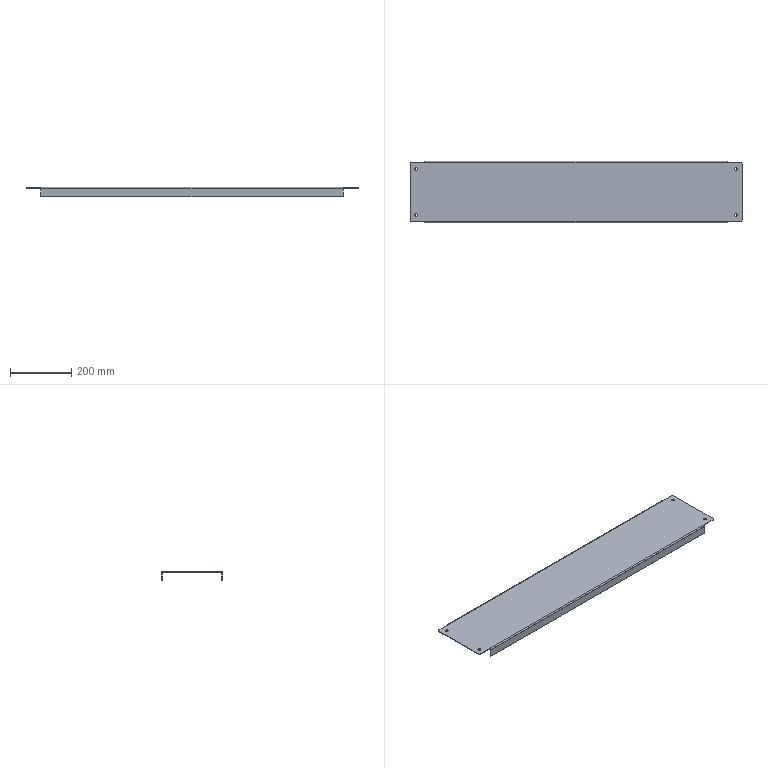Part | STEP file | 750038142 | 1 solid | 34 faces | box 1086 x 200 x 30 mm | volume 538093 mm3 | plane 18 | cylinder 16 | commonest cylinder face diameters 9 x8 10 x4 4 x2 8 x2
STEP:
#1=CARTESIAN_POINT('',(-527.5,-75.,0.));
#2=VERTEX_POINT('',#1);
#3=CARTESIAN_POINT('',(-518.5,-75.,0.));
#4=VERTEX_POINT('',#3);
#5=CARTESIAN_POINT('',(-523.,-75.,0.));
#6=DIRECTION('',(0.,0.,1.));
#7=DIRECTION('',(1.,0.,0.));
#8=AXIS2_PLACEMENT_3D('',#5,#6,#7);
#9=CIRCLE('',#8,4.5);
#10=EDGE_CURVE('',#2,#4,#9,.T.);
#11=ORIENTED_EDGE('',*,*,#10,.F.);
#12=CARTESIAN_POINT('',(-527.5,-75.,2.));
#13=VERTEX_POINT('',#12);
#14=CARTESIAN_POINT('',(-527.5,-75.,-1102.67));
#15=DIRECTION('',(0.,0.,1.));
#16=VECTOR('',#15,1000.);
#17=LINE('',#14,#16);
#18=EDGE_CURVE('',#2,#13,#17,.T.);
#19=ORIENTED_EDGE('',*,*,#18,.T.);
#20=CARTESIAN_POINT('',(-518.5,-75.,2.));
#21=VERTEX_POINT('',#20);
#22=CARTESIAN_POINT('',(-523.,-75.,2.));
#23=DIRECTION('',(0.,0.,-1.));
#24=DIRECTION('',(1.,0.,0.));
#25=AXIS2_PLACEMENT_3D('',#22,#23,#24);
#26=CIRCLE('',#25,4.5);
#27=EDGE_CURVE('',#21,#13,#26,.T.);
#28=ORIENTED_EDGE('',*,*,#27,.F.);
#29=CARTESIAN_POINT('',(-518.5,-75.,-1102.67));
#30=DIRECTION('',(0.,0.,1.));
#31=VECTOR('',#30,1000.);
#32=LINE('',#29,#31);
#33=EDGE_CURVE('',#4,#21,#32,.T.);
#34=ORIENTED_EDGE('',*,*,#33,.F.);
#35=EDGE_LOOP('',(#11,#19,#28,#34));
#36=FACE_OUTER_BOUND('',#35,.T.);
#37=CARTESIAN_POINT('',(-523.,-75.,-1102.67));
#38=DIRECTION('',(0.,0.,1.));
#39=DIRECTION('',(1.,0.,0.));
#40=AXIS2_PLACEMENT_3D('',#37,#38,#39);
#41=CYLINDRICAL_SURFACE('',#40,4.5);
#42=ADVANCED_FACE('',(#36),#41,.F.);
#43=CARTESIAN_POINT('',(-527.5,75.,0.));
#44=VERTEX_POINT('',#43);
#45=CARTESIAN_POINT('',(-518.5,75.,0.));
#46=VERTEX_POINT('',#45);
#47=CARTESIAN_POINT('',(-523.,75.,0.));
#48=DIRECTION('',(0.,0.,1.));
#49=DIRECTION('',(1.,0.,0.));
#50=AXIS2_PLACEMENT_3D('',#47,#48,#49);
#51=CIRCLE('',#50,4.5);
#52=EDGE_CURVE('',#44,#46,#51,.T.);
#53=ORIENTED_EDGE('',*,*,#52,.F.);
#54=CARTESIAN_POINT('',(-527.5,75.,2.));
#55=VERTEX_POINT('',#54);
#56=CARTESIAN_POINT('',(-527.5,75.,-1102.67));
#57=DIRECTION('',(0.,0.,1.));
#58=VECTOR('',#57,1000.);
#59=LINE('',#56,#58);
#60=EDGE_CURVE('',#44,#55,#59,.T.);
#61=ORIENTED_EDGE('',*,*,#60,.T.);
#62=CARTESIAN_POINT('',(-518.5,75.,2.));
#63=VERTEX_POINT('',#62);
#64=CARTESIAN_POINT('',(-523.,75.,2.));
#65=DIRECTION('',(0.,0.,-1.));
#66=DIRECTION('',(1.,0.,0.));
#67=AXIS2_PLACEMENT_3D('',#64,#65,#66);
#68=CIRCLE('',#67,4.5);
#69=EDGE_CURVE('',#63,#55,#68,.T.);
#70=ORIENTED_EDGE('',*,*,#69,.F.);
#71=CARTESIAN_POINT('',(-518.5,75.,-1102.67));
#72=DIRECTION('',(0.,0.,1.));
#73=VECTOR('',#72,1000.);
#74=LINE('',#71,#73);
#75=EDGE_CURVE('',#46,#63,#74,.T.);
#76=ORIENTED_EDGE('',*,*,#75,.F.);
#77=EDGE_LOOP('',(#53,#61,#70,#76));
#78=FACE_OUTER_BOUND('',#77,.T.);
#79=CARTESIAN_POINT('',(-523.,75.,-1102.67));
#80=DIRECTION('',(0.,0.,1.));
#81=DIRECTION('',(1.,0.,0.));
#82=AXIS2_PLACEMENT_3D('',#79,#80,#81);
#83=CYLINDRICAL_SURFACE('',#82,4.5);
#84=ADVANCED_FACE('',(#78),#83,.F.);
#85=CARTESIAN_POINT('',(518.5,-75.,0.));
#86=VERTEX_POINT('',#85);
#87=CARTESIAN_POINT('',(527.5,-75.,0.));
#88=VERTEX_POINT('',#87);
#89=CARTESIAN_POINT('',(523.,-75.,0.));
#90=DIRECTION('',(0.,0.,1.));
#91=DIRECTION('',(1.,0.,0.));
#92=AXIS2_PLACEMENT_3D('',#89,#90,#91);
#93=CIRCLE('',#92,4.5);
#94=EDGE_CURVE('',#86,#88,#93,.T.);
#95=ORIENTED_EDGE('',*,*,#94,.F.);
#96=CARTESIAN_POINT('',(518.5,-75.,2.));
#97=VERTEX_POINT('',#96);
#98=CARTESIAN_POINT('',(518.5,-75.,-1102.67));
#99=DIRECTION('',(0.,0.,1.));
#100=VECTOR('',#99,1000.);
#101=LINE('',#98,#100);
#102=EDGE_CURVE('',#86,#97,#101,.T.);
#103=ORIENTED_EDGE('',*,*,#102,.T.);
#104=CARTESIAN_POINT('',(527.5,-75.,2.));
#105=VERTEX_POINT('',#104);
#106=CARTESIAN_POINT('',(523.,-75.,2.));
#107=DIRECTION('',(0.,0.,-1.));
#108=DIRECTION('',(1.,0.,0.));
#109=AXIS2_PLACEMENT_3D('',#106,#107,#108);
#110=CIRCLE('',#109,4.5);
#111=EDGE_CURVE('',#105,#97,#110,.T.);
#112=ORIENTED_EDGE('',*,*,#111,.F.);
#113=CARTESIAN_POINT('',(527.5,-75.,-1102.67));
#114=DIRECTION('',(0.,0.,1.));
#115=VECTOR('',#114,1000.);
#116=LINE('',#113,#115);
#117=EDGE_CURVE('',#88,#105,#116,.T.);
#118=ORIENTED_EDGE('',*,*,#117,.F.);
#119=EDGE_LOOP('',(#95,#103,#112,#118));
#120=FACE_OUTER_BOUND('',#119,.T.);
#121=CARTESIAN_POINT('',(523.,-75.,-1102.67));
#122=DIRECTION('',(0.,0.,1.));
#123=DIRECTION('',(1.,0.,0.));
#124=AXIS2_PLACEMENT_3D('',#121,#122,#123);
#125=CYLINDRICAL_SURFACE('',#124,4.5);
#126=ADVANCED_FACE('',(#120),#125,.F.);
#127=CARTESIAN_POINT('',(518.5,75.,0.));
#128=VERTEX_POINT('',#127);
#129=CARTESIAN_POINT('',(527.5,75.,0.));
#130=VERTEX_POINT('',#129);
#131=CARTESIAN_POINT('',(523.,75.,0.));
#132=DIRECTION('',(0.,0.,1.));
#133=DIRECTION('',(1.,0.,0.));
#134=AXIS2_PLACEMENT_3D('',#131,#132,#133);
#135=CIRCLE('',#134,4.5);
#136=EDGE_CURVE('',#128,#130,#135,.T.);
#137=ORIENTED_EDGE('',*,*,#136,.F.);
#138=CARTESIAN_POINT('',(518.5,75.,2.));
#139=VERTEX_POINT('',#138);
#140=CARTESIAN_POINT('',(518.5,75.,-1102.67));
#141=DIRECTION('',(0.,0.,1.));
#142=VECTOR('',#141,1000.);
#143=LINE('',#140,#142);
#144=EDGE_CURVE('',#128,#139,#143,.T.);
#145=ORIENTED_EDGE('',*,*,#144,.T.);
#146=CARTESIAN_POINT('',(527.5,75.,2.));
#147=VERTEX_POINT('',#146);
#148=CARTESIAN_POINT('',(523.,75.,2.));
#149=DIRECTION('',(0.,0.,-1.));
#150=DIRECTION('',(1.,0.,0.));
#151=AXIS2_PLACEMENT_3D('',#148,#149,#150);
#152=CIRCLE('',#151,4.5);
#153=EDGE_CURVE('',#147,#139,#152,.T.);
#154=ORIENTED_EDGE('',*,*,#153,.F.);
#155=CARTESIAN_POINT('',(527.5,75.,-1102.67));
#156=DIRECTION('',(0.,0.,1.));
#157=VECTOR('',#156,1000.);
#158=LINE('',#155,#157);
#159=EDGE_CURVE('',#130,#147,#158,.T.);
#160=ORIENTED_EDGE('',*,*,#159,.F.);
#161=EDGE_LOOP('',(#137,#145,#154,#160));
#162=FACE_OUTER_BOUND('',#161,.T.);
#163=CARTESIAN_POINT('',(523.,75.,-1102.67));
#164=DIRECTION('',(0.,0.,1.));
#165=DIRECTION('',(1.,0.,0.));
#166=AXIS2_PLACEMENT_3D('',#163,#164,#165);
#167=CYLINDRICAL_SURFACE('',#166,4.5);
#168=ADVANCED_FACE('',(#162),#167,.F.);
#169=CARTESIAN_POINT('',(538.,96.,2.));
#170=VERTEX_POINT('',#169);
#171=CARTESIAN_POINT('',(495.,96.,2.));
#172=VERTEX_POINT('',#171);
#173=CARTESIAN_POINT('',(0.,96.,2.));
#174=DIRECTION('',(-1.,0.,0.));
#175=VECTOR('',#174,1000.);
#176=LINE('',#173,#175);
#177=EDGE_CURVE('',#170,#172,#176,.T.);
#178=ORIENTED_EDGE('',*,*,#177,.T.);
#179=CARTESIAN_POINT('',(-495.,96.,2.));
#180=VERTEX_POINT('',#179);
#181=CARTESIAN_POINT('',(0.,96.,2.));
#182=DIRECTION('',(-1.,0.,0.));
#183=VECTOR('',#182,1000.);
#184=LINE('',#181,#183);
#185=EDGE_CURVE('',#172,#180,#184,.T.);
#186=ORIENTED_EDGE('',*,*,#185,.T.);
#187=CARTESIAN_POINT('',(-538.,96.,2.));
#188=VERTEX_POINT('',#187);
#189=CARTESIAN_POINT('',(0.,96.,2.));
#190=DIRECTION('',(-1.,0.,0.));
#191=VECTOR('',#190,1000.);
#192=LINE('',#189,#191);
#193=EDGE_CURVE('',#180,#188,#192,.T.);
#194=ORIENTED_EDGE('',*,*,#193,.T.);
#195=CARTESIAN_POINT('',(-543.,91.,2.));
#196=VERTEX_POINT('',#195);
#197=CARTESIAN_POINT('',(-538.,91.,2.));
#198=DIRECTION('',(0.,0.,1.));
#199=DIRECTION('',(-1.,0.,0.));
#200=AXIS2_PLACEMENT_3D('',#197,#198,#199);
#201=CIRCLE('',#200,5.);
#202=EDGE_CURVE('',#188,#196,#201,.T.);
#203=ORIENTED_EDGE('',*,*,#202,.T.);
#204=CARTESIAN_POINT('',(-543.,-91.,2.));
#205=VERTEX_POINT('',#204);
#206=CARTESIAN_POINT('',(-543.,0.,2.));
#207=DIRECTION('',(0.,-1.,0.));
#208=VECTOR('',#207,1000.);
#209=LINE('',#206,#208);
#210=EDGE_CURVE('',#196,#205,#209,.T.);
#211=ORIENTED_EDGE('',*,*,#210,.T.);
#212=CARTESIAN_POINT('',(-538.,-96.,2.));
#213=VERTEX_POINT('',#212);
#214=CARTESIAN_POINT('',(-538.,-91.,2.));
#215=DIRECTION('',(0.,0.,1.));
#216=DIRECTION('',(-1.,0.,0.));
#217=AXIS2_PLACEMENT_3D('',#214,#215,#216);
#218=CIRCLE('',#217,5.);
#219=EDGE_CURVE('',#205,#213,#218,.T.);
#220=ORIENTED_EDGE('',*,*,#219,.T.);
#221=CARTESIAN_POINT('',(-495.,-96.,2.));
#222=VERTEX_POINT('',#221);
#223=CARTESIAN_POINT('',(0.,-96.,2.));
#224=DIRECTION('',(1.,0.,0.));
#225=VECTOR('',#224,1000.);
#226=LINE('',#223,#225);
#227=EDGE_CURVE('',#213,#222,#226,.T.);
#228=ORIENTED_EDGE('',*,*,#227,.T.);
#229=CARTESIAN_POINT('',(495.,-96.,2.));
#230=VERTEX_POINT('',#229);
#231=CARTESIAN_POINT('',(0.,-96.,2.));
#232=DIRECTION('',(1.,0.,0.));
#233=VECTOR('',#232,1000.);
#234=LINE('',#231,#233);
#235=EDGE_CURVE('',#222,#230,#234,.T.);
#236=ORIENTED_EDGE('',*,*,#235,.T.);
#237=CARTESIAN_POINT('',(538.,-96.,2.));
#238=VERTEX_POINT('',#237);
#239=CARTESIAN_POINT('',(0.,-96.,2.));
#240=DIRECTION('',(1.,0.,0.));
#241=VECTOR('',#240,1000.);
#242=LINE('',#239,#241);
#243=EDGE_CURVE('',#230,#238,#242,.T.);
#244=ORIENTED_EDGE('',*,*,#243,.T.);
#245=CARTESIAN_POINT('',(543.,-91.,2.));
#246=VERTEX_POINT('',#245);
#247=CARTESIAN_POINT('',(538.,-91.,2.));
#248=DIRECTION('',(0.,0.,1.));
#249=DIRECTION('',(-1.,0.,0.));
#250=AXIS2_PLACEMENT_3D('',#247,#248,#249);
#251=CIRCLE('',#250,5.);
#252=EDGE_CURVE('',#238,#246,#251,.T.);
#253=ORIENTED_EDGE('',*,*,#252,.T.);
#254=CARTESIAN_POINT('',(543.,91.,2.));
#255=VERTEX_POINT('',#254);
#256=CARTESIAN_POINT('',(543.,0.,2.));
#257=DIRECTION('',(0.,1.,0.));
#258=VECTOR('',#257,1000.);
#259=LINE('',#256,#258);
#260=EDGE_CURVE('',#246,#255,#259,.T.);
#261=ORIENTED_EDGE('',*,*,#260,.T.);
#262=CARTESIAN_POINT('',(538.,91.,2.));
#263=DIRECTION('',(0.,0.,1.));
#264=DIRECTION('',(-1.,0.,0.));
#265=AXIS2_PLACEMENT_3D('',#262,#263,#264);
#266=CIRCLE('',#265,5.);
#267=EDGE_CURVE('',#255,#170,#266,.T.);
#268=ORIENTED_EDGE('',*,*,#267,.T.);
#269=EDGE_LOOP('',(#178,#186,#194,#203,#211,#220,#228,#236,#244,#253,#261,#268));
#270=FACE_OUTER_BOUND('',#269,.T.);
#271=ORIENTED_EDGE('',*,*,#27,.T.);
#272=CARTESIAN_POINT('',(-523.,-75.,2.));
#273=DIRECTION('',(0.,0.,-1.));
#274=DIRECTION('',(1.,0.,0.));
#275=AXIS2_PLACEMENT_3D('',#272,#273,#274);
#276=CIRCLE('',#275,4.5);
#277=EDGE_CURVE('',#13,#21,#276,.T.);
#278=ORIENTED_EDGE('',*,*,#277,.T.);
#279=EDGE_LOOP('',(#271,#278));
#280=FACE_BOUND('',#279,.T.);
#281=ORIENTED_EDGE('',*,*,#69,.T.);
#282=CARTESIAN_POINT('',(-523.,75.,2.));
#283=DIRECTION('',(0.,0.,-1.));
#284=DIRECTION('',(1.,0.,0.));
#285=AXIS2_PLACEMENT_3D('',#282,#283,#284);
#286=CIRCLE('',#285,4.5);
#287=EDGE_CURVE('',#55,#63,#286,.T.);
#288=ORIENTED_EDGE('',*,*,#287,.T.);
#289=EDGE_LOOP('',(#281,#288));
#290=FACE_BOUND('',#289,.T.);
#291=ORIENTED_EDGE('',*,*,#111,.T.);
#292=CARTESIAN_POINT('',(523.,-75.,2.));
#293=DIRECTION('',(0.,0.,-1.));
#294=DIRECTION('',(1.,0.,0.));
#295=AXIS2_PLACEMENT_3D('',#292,#293,#294);
#296=CIRCLE('',#295,4.5);
#297=EDGE_CURVE('',#97,#105,#296,.T.);
#298=ORIENTED_EDGE('',*,*,#297,.T.);
#299=EDGE_LOOP('',(#291,#298));
#300=FACE_BOUND('',#299,.T.);
#301=ORIENTED_EDGE('',*,*,#153,.T.);
#302=CARTESIAN_POINT('',(523.,75.,2.));
#303=DIRECTION('',(0.,0.,-1.));
#304=DIRECTION('',(1.,0.,0.));
#305=AXIS2_PLACEMENT_3D('',#302,#303,#304);
#306=CIRCLE('',#305,4.5);
#307=EDGE_CURVE('',#139,#147,#306,.T.);
#308=ORIENTED_EDGE('',*,*,#307,.T.);
#309=EDGE_LOOP('',(#301,#308));
#310=FACE_BOUND('',#309,.T.);
#311=CARTESIAN_POINT('',(0.,0.,2.));
#312=DIRECTION('',(0.,0.,1.));
#313=DIRECTION('',(1.,0.,0.));
#314=AXIS2_PLACEMENT_3D('',#311,#312,#313);
#315=PLANE('',#314);
#316=ADVANCED_FACE('',(#270,#280,#290,#300,#310),#315,.T.);
#317=CARTESIAN_POINT('',(-495.,100.,-2.));
#318=VERTEX_POINT('',#317);
#319=CARTESIAN_POINT('',(-495.,96.,-2.));
#320=DIRECTION('',(1.,0.,0.));
#321=DIRECTION('',(0.,0.,-1.));
#322=AXIS2_PLACEMENT_3D('',#319,#320,#321);
#323=CIRCLE('',#322,4.);
#324=EDGE_CURVE('',#318,#180,#323,.T.);
#325=ORIENTED_EDGE('',*,*,#324,.T.);
#326=ORIENTED_EDGE('',*,*,#185,.F.);
#327=CARTESIAN_POINT('',(495.,100.,-2.));
#328=VERTEX_POINT('',#327);
#329=CARTESIAN_POINT('',(495.,96.,-2.));
#330=DIRECTION('',(-1.,0.,0.));
#331=DIRECTION('',(0.,0.,-1.));
#332=AXIS2_PLACEMENT_3D('',#329,#330,#331);
#333=CIRCLE('',#332,4.);
#334=EDGE_CURVE('',#172,#328,#333,.T.);
#335=ORIENTED_EDGE('',*,*,#334,.T.);
#336=CARTESIAN_POINT('',(-495.,100.,-2.));
#337=DIRECTION('',(-1.,0.,0.));
#338=VECTOR('',#337,1000.);
#339=LINE('',#336,#338);
#340=EDGE_CURVE('',#328,#318,#339,.T.);
#341=ORIENTED_EDGE('',*,*,#340,.T.);
#342=EDGE_LOOP('',(#325,#326,#335,#341));
#343=FACE_OUTER_BOUND('',#342,.T.);
#344=CARTESIAN_POINT('',(-495.,96.,-2.));
#345=DIRECTION('',(1.,0.,0.));
#346=DIRECTION('',(0.,0.,-1.));
#347=AXIS2_PLACEMENT_3D('',#344,#345,#346);
#348=CYLINDRICAL_SURFACE('',#347,4.);
#349=ADVANCED_FACE('',(#343),#348,.T.);
#350=CARTESIAN_POINT('',(538.,96.,0.));
#351=VERTEX_POINT('',#350);
#352=CARTESIAN_POINT('',(538.,96.,2.));
#353=DIRECTION('',(0.,0.,1.));
#354=VECTOR('',#353,1000.);
#355=LINE('',#352,#354);
#356=EDGE_CURVE('',#351,#170,#355,.T.);
#357=ORIENTED_EDGE('',*,*,#356,.F.);
#358=CARTESIAN_POINT('',(495.,96.,0.));
#359=VERTEX_POINT('',#358);
#360=CARTESIAN_POINT('',(543.,96.,0.));
#361=DIRECTION('',(1.,0.,0.));
#362=VECTOR('',#361,1000.);
#363=LINE('',#360,#362);
#364=EDGE_CURVE('',#359,#351,#363,.T.);
#365=ORIENTED_EDGE('',*,*,#364,.F.);
#366=CARTESIAN_POINT('',(495.,96.,2.));
#367=DIRECTION('',(0.,0.,-1.));
#368=VECTOR('',#367,1000.);
#369=LINE('',#366,#368);
#370=EDGE_CURVE('',#172,#359,#369,.T.);
#371=ORIENTED_EDGE('',*,*,#370,.F.);
#372=ORIENTED_EDGE('',*,*,#177,.F.);
#373=EDGE_LOOP('',(#357,#365,#371,#372));
#374=FACE_OUTER_BOUND('',#373,.T.);
#375=CARTESIAN_POINT('',(543.,96.,2.));
#376=DIRECTION('',(0.,-1.,0.));
#377=DIRECTION('',(0.,0.,-1.));
#378=AXIS2_PLACEMENT_3D('',#375,#376,#377);
#379=PLANE('',#378);
#380=ADVANCED_FACE('',(#374),#379,.F.);
#381=CARTESIAN_POINT('',(543.,91.,0.));
#382=VERTEX_POINT('',#381);
#383=CARTESIAN_POINT('',(538.,91.,0.));
#384=DIRECTION('',(0.,0.,1.));
#385=DIRECTION('',(-1.,0.,0.));
#386=AXIS2_PLACEMENT_3D('',#383,#384,#385);
#387=CIRCLE('',#386,5.);
#388=EDGE_CURVE('',#382,#351,#387,.T.);
#389=ORIENTED_EDGE('',*,*,#388,.T.);
#390=ORIENTED_EDGE('',*,*,#356,.T.);
#391=ORIENTED_EDGE('',*,*,#267,.F.);
#392=CARTESIAN_POINT('',(543.,91.,2.));
#393=DIRECTION('',(0.,0.,-1.));
#394=VECTOR('',#393,1000.);
#395=LINE('',#392,#394);
#396=EDGE_CURVE('',#255,#382,#395,.T.);
#397=ORIENTED_EDGE('',*,*,#396,.T.);
#398=EDGE_LOOP('',(#389,#390,#391,#397));
#399=FACE_OUTER_BOUND('',#398,.T.);
#400=CARTESIAN_POINT('',(538.,91.,2.));
#401=DIRECTION('',(0.,0.,-1.));
#402=DIRECTION('',(-1.,0.,0.));
#403=AXIS2_PLACEMENT_3D('',#400,#401,#402);
#404=CYLINDRICAL_SURFACE('',#403,5.);
#405=ADVANCED_FACE('',(#399),#404,.T.);
#406=CARTESIAN_POINT('',(543.,-91.,0.));
#407=VERTEX_POINT('',#406);
#408=CARTESIAN_POINT('',(543.,-91.,2.));
#409=DIRECTION('',(0.,0.,1.));
#410=VECTOR('',#409,1000.);
#411=LINE('',#408,#410);
#412=EDGE_CURVE('',#407,#246,#411,.T.);
#413=ORIENTED_EDGE('',*,*,#412,.F.);
#414=CARTESIAN_POINT('',(543.,-96.,0.));
#415=DIRECTION('',(0.,-1.,0.));
#416=VECTOR('',#415,1000.);
#417=LINE('',#414,#416);
#418=EDGE_CURVE('',#382,#407,#417,.T.);
#419=ORIENTED_EDGE('',*,*,#418,.F.);
#420=ORIENTED_EDGE('',*,*,#396,.F.);
#421=ORIENTED_EDGE('',*,*,#260,.F.);
#422=EDGE_LOOP('',(#413,#419,#420,#421));
#423=FACE_OUTER_BOUND('',#422,.T.);
#424=CARTESIAN_POINT('',(543.,-96.,2.));
#425=DIRECTION('',(-1.,0.,0.));
#426=DIRECTION('',(0.,0.,1.));
#427=AXIS2_PLACEMENT_3D('',#424,#425,#426);
#428=PLANE('',#427);
#429=ADVANCED_FACE('',(#423),#428,.F.);
#430=CARTESIAN_POINT('',(538.,-96.,0.));
#431=VERTEX_POINT('',#430);
#432=CARTESIAN_POINT('',(538.,-91.,0.));
#433=DIRECTION('',(0.,0.,1.));
#434=DIRECTION('',(-1.,0.,0.));
#435=AXIS2_PLACEMENT_3D('',#432,#433,#434);
#436=CIRCLE('',#435,5.);
#437=EDGE_CURVE('',#431,#407,#436,.T.);
#438=ORIENTED_EDGE('',*,*,#437,.T.);
#439=ORIENTED_EDGE('',*,*,#412,.T.);
#440=ORIENTED_EDGE('',*,*,#252,.F.);
#441=CARTESIAN_POINT('',(538.,-96.,2.));
#442=DIRECTION('',(0.,0.,-1.));
#443=VECTOR('',#442,1000.);
#444=LINE('',#441,#443);
#445=EDGE_CURVE('',#238,#431,#444,.T.);
#446=ORIENTED_EDGE('',*,*,#445,.T.);
#447=EDGE_LOOP('',(#438,#439,#440,#446));
#448=FACE_OUTER_BOUND('',#447,.T.);
#449=CARTESIAN_POINT('',(538.,-91.,2.));
#450=DIRECTION('',(0.,0.,-1.));
#451=DIRECTION('',(-1.,0.,0.));
#452=AXIS2_PLACEMENT_3D('',#449,#450,#451);
#453=CYLINDRICAL_SURFACE('',#452,5.);
#454=ADVANCED_FACE('',(#448),#453,.T.);
#455=ORIENTED_EDGE('',*,*,#445,.F.);
#456=ORIENTED_EDGE('',*,*,#243,.F.);
#457=CARTESIAN_POINT('',(495.,-96.,0.));
#458=VERTEX_POINT('',#457);
#459=CARTESIAN_POINT('',(495.,-96.,2.));
#460=DIRECTION('',(0.,0.,1.));
#461=VECTOR('',#460,1000.);
#462=LINE('',#459,#461);
#463=EDGE_CURVE('',#458,#230,#462,.T.);
#464=ORIENTED_EDGE('',*,*,#463,.F.);
#465=CARTESIAN_POINT('',(-543.,-96.,0.));
#466=DIRECTION('',(-1.,0.,0.));
#467=VECTOR('',#466,1000.);
#468=LINE('',#465,#467);
#469=EDGE_CURVE('',#431,#458,#468,.T.);
#470=ORIENTED_EDGE('',*,*,#469,.F.);
#471=EDGE_LOOP('',(#455,#456,#464,#470));
#472=FACE_OUTER_BOUND('',#471,.T.);
#473=CARTESIAN_POINT('',(-543.,-96.,2.));
#474=DIRECTION('',(0.,1.,0.));
#475=DIRECTION('',(0.,0.,1.));
#476=AXIS2_PLACEMENT_3D('',#473,#474,#475);
#477=PLANE('',#476);
#478=ADVANCED_FACE('',(#472),#477,.F.);
#479=CARTESIAN_POINT('',(495.,-100.,-2.));
#480=VERTEX_POINT('',#479);
#481=CARTESIAN_POINT('',(495.,-96.,-2.));
#482=DIRECTION('',(-1.,0.,0.));
#483=DIRECTION('',(0.,0.,1.));
#484=AXIS2_PLACEMENT_3D('',#481,#482,#483);
#485=CIRCLE('',#484,4.);
#486=EDGE_CURVE('',#480,#230,#485,.T.);
#487=ORIENTED_EDGE('',*,*,#486,.T.);
#488=ORIENTED_EDGE('',*,*,#235,.F.);
#489=CARTESIAN_POINT('',(-495.,-100.,-2.));
#490=VERTEX_POINT('',#489);
#491=CARTESIAN_POINT('',(-495.,-96.,-2.));
#492=DIRECTION('',(1.,0.,0.));
#493=DIRECTION('',(0.,0.,1.));
#494=AXIS2_PLACEMENT_3D('',#491,#492,#493);
#495=CIRCLE('',#494,4.);
#496=EDGE_CURVE('',#222,#490,#495,.T.);
#497=ORIENTED_EDGE('',*,*,#496,.T.);
#498=CARTESIAN_POINT('',(495.,-100.,-2.));
#499=DIRECTION('',(1.,0.,0.));
#500=VECTOR('',#499,1000.);
#501=LINE('',#498,#500);
#502=EDGE_CURVE('',#490,#480,#501,.T.);
#503=ORIENTED_EDGE('',*,*,#502,.T.);
#504=EDGE_LOOP('',(#487,#488,#497,#503));
#505=FACE_OUTER_BOUND('',#504,.T.);
#506=CARTESIAN_POINT('',(495.,-96.,-2.));
#507=DIRECTION('',(-1.,0.,0.));
#508=DIRECTION('',(0.,0.,1.));
#509=AXIS2_PLACEMENT_3D('',#506,#507,#508);
#510=CYLINDRICAL_SURFACE('',#509,4.);
#511=ADVANCED_FACE('',(#505),#510,.T.);
#512=CARTESIAN_POINT('',(-538.,-96.,0.));
#513=VERTEX_POINT('',#512);
#514=CARTESIAN_POINT('',(-538.,-96.,2.));
#515=DIRECTION('',(0.,0.,1.));
#516=VECTOR('',#515,1000.);
#517=LINE('',#514,#516);
#518=EDGE_CURVE('',#513,#213,#517,.T.);
#519=ORIENTED_EDGE('',*,*,#518,.F.);
#520=CARTESIAN_POINT('',(-495.,-96.,0.));
#521=VERTEX_POINT('',#520);
#522=CARTESIAN_POINT('',(-543.,-96.,0.));
#523=DIRECTION('',(-1.,0.,0.));
#524=VECTOR('',#523,1000.);
#525=LINE('',#522,#524);
#526=EDGE_CURVE('',#521,#513,#525,.T.);
#527=ORIENTED_EDGE('',*,*,#526,.F.);
#528=CARTESIAN_POINT('',(-495.,-96.,2.));
#529=DIRECTION('',(0.,0.,-1.));
#530=VECTOR('',#529,1000.);
#531=LINE('',#528,#530);
#532=EDGE_CURVE('',#222,#521,#531,.T.);
#533=ORIENTED_EDGE('',*,*,#532,.F.);
#534=ORIENTED_EDGE('',*,*,#227,.F.);
#535=EDGE_LOOP('',(#519,#527,#533,#534));
#536=FACE_OUTER_BOUND('',#535,.T.);
#537=CARTESIAN_POINT('',(-543.,-96.,2.));
#538=DIRECTION('',(0.,1.,0.));
#539=DIRECTION('',(0.,0.,1.));
#540=AXIS2_PLACEMENT_3D('',#537,#538,#539);
#541=PLANE('',#540);
#542=ADVANCED_FACE('',(#536),#541,.F.);
#543=CARTESIAN_POINT('',(-543.,-91.,0.));
#544=VERTEX_POINT('',#543);
#545=CARTESIAN_POINT('',(-538.,-91.,0.));
#546=DIRECTION('',(0.,0.,1.));
#547=DIRECTION('',(-1.,0.,0.));
#548=AXIS2_PLACEMENT_3D('',#545,#546,#547);
#549=CIRCLE('',#548,5.);
#550=EDGE_CURVE('',#544,#513,#549,.T.);
#551=ORIENTED_EDGE('',*,*,#550,.T.);
#552=ORIENTED_EDGE('',*,*,#518,.T.);
#553=ORIENTED_EDGE('',*,*,#219,.F.);
#554=CARTESIAN_POINT('',(-543.,-91.,2.));
#555=DIRECTION('',(0.,0.,-1.));
#556=VECTOR('',#555,1000.);
#557=LINE('',#554,#556);
#558=EDGE_CURVE('',#205,#544,#557,.T.);
#559=ORIENTED_EDGE('',*,*,#558,.T.);
#560=EDGE_LOOP('',(#551,#552,#553,#559));
#561=FACE_OUTER_BOUND('',#560,.T.);
#562=CARTESIAN_POINT('',(-538.,-91.,2.));
#563=DIRECTION('',(0.,0.,-1.));
#564=DIRECTION('',(-1.,0.,0.));
#565=AXIS2_PLACEMENT_3D('',#562,#563,#564);
#566=CYLINDRICAL_SURFACE('',#565,5.);
#567=ADVANCED_FACE('',(#561),#566,.T.);
#568=CARTESIAN_POINT('',(-543.,91.,0.));
#569=VERTEX_POINT('',#568);
#570=CARTESIAN_POINT('',(-543.,91.,2.));
#571=DIRECTION('',(0.,0.,1.));
#572=VECTOR('',#571,1000.);
#573=LINE('',#570,#572);
#574=EDGE_CURVE('',#569,#196,#573,.T.);
#575=ORIENTED_EDGE('',*,*,#574,.F.);
#576=CARTESIAN_POINT('',(-543.,96.,0.));
#577=DIRECTION('',(0.,1.,0.));
#578=VECTOR('',#577,1000.);
#579=LINE('',#576,#578);
#580=EDGE_CURVE('',#544,#569,#579,.T.);
#581=ORIENTED_EDGE('',*,*,#580,.F.);
#582=ORIENTED_EDGE('',*,*,#558,.F.);
#583=ORIENTED_EDGE('',*,*,#210,.F.);
#584=EDGE_LOOP('',(#575,#581,#582,#583));
#585=FACE_OUTER_BOUND('',#584,.T.);
#586=CARTESIAN_POINT('',(-543.,96.,2.));
#587=DIRECTION('',(1.,0.,0.));
#588=DIRECTION('',(0.,0.,-1.));
#589=AXIS2_PLACEMENT_3D('',#586,#587,#588);
#590=PLANE('',#589);
#591=ADVANCED_FACE('',(#585),#590,.F.);
#592=CARTESIAN_POINT('',(-538.,96.,0.));
#593=VERTEX_POINT('',#592);
#594=CARTESIAN_POINT('',(-538.,91.,0.));
#595=DIRECTION('',(0.,0.,1.));
#596=DIRECTION('',(-1.,0.,0.));
#597=AXIS2_PLACEMENT_3D('',#594,#595,#596);
#598=CIRCLE('',#597,5.);
#599=EDGE_CURVE('',#593,#569,#598,.T.);
#600=ORIENTED_EDGE('',*,*,#599,.T.);
#601=ORIENTED_EDGE('',*,*,#574,.T.);
#602=ORIENTED_EDGE('',*,*,#202,.F.);
#603=CARTESIAN_POINT('',(-538.,96.,2.));
#604=DIRECTION('',(0.,0.,-1.));
#605=VECTOR('',#604,1000.);
#606=LINE('',#603,#605);
#607=EDGE_CURVE('',#188,#593,#606,.T.);
#608=ORIENTED_EDGE('',*,*,#607,.T.);
#609=EDGE_LOOP('',(#600,#601,#602,#608));
#610=FACE_OUTER_BOUND('',#609,.T.);
#611=CARTESIAN_POINT('',(-538.,91.,2.));
#612=DIRECTION('',(0.,0.,-1.));
#613=DIRECTION('',(-1.,0.,0.));
#614=AXIS2_PLACEMENT_3D('',#611,#612,#613);
#615=CYLINDRICAL_SURFACE('',#614,5.);
#616=ADVANCED_FACE('',(#610),#615,.T.);
#617=ORIENTED_EDGE('',*,*,#607,.F.);
#618=ORIENTED_EDGE('',*,*,#193,.F.);
#619=CARTESIAN_POINT('',(-495.,96.,0.));
#620=VERTEX_POINT('',#619);
#621=CARTESIAN_POINT('',(-495.,96.,2.));
#622=DIRECTION('',(0.,0.,1.));
#623=VECTOR('',#622,1000.);
#624=LINE('',#621,#623);
#625=EDGE_CURVE('',#620,#180,#624,.T.);
#626=ORIENTED_EDGE('',*,*,#625,.F.);
#627=CARTESIAN_POINT('',(543.,96.,0.));
#628=DIRECTION('',(1.,0.,0.));
#629=VECTOR('',#628,1000.);
#630=LINE('',#627,#629);
#631=EDGE_CURVE('',#593,#620,#630,.T.);
#632=ORIENTED_EDGE('',*,*,#631,.F.);
#633=EDGE_LOOP('',(#617,#618,#626,#632));
#634=FACE_OUTER_BOUND('',#633,.T.);
#635=CARTESIAN_POINT('',(543.,96.,2.));
#636=DIRECTION('',(0.,-1.,0.));
#637=DIRECTION('',(0.,0.,-1.));
#638=AXIS2_PLACEMENT_3D('',#635,#636,#637);
#639=PLANE('',#638);
#640=ADVANCED_FACE('',(#634),#639,.F.);
#641=ORIENTED_EDGE('',*,*,#18,.F.);
#642=CARTESIAN_POINT('',(-523.,-75.,0.));
#643=DIRECTION('',(0.,0.,1.));
#644=DIRECTION('',(1.,0.,0.));
#645=AXIS2_PLACEMENT_3D('',#642,#643,#644);
#646=CIRCLE('',#645,4.5);
#647=EDGE_CURVE('',#4,#2,#646,.T.);
#648=ORIENTED_EDGE('',*,*,#647,.F.);
#649=ORIENTED_EDGE('',*,*,#33,.T.);
#650=ORIENTED_EDGE('',*,*,#277,.F.);
#651=EDGE_LOOP('',(#641,#648,#649,#650));
#652=FACE_OUTER_BOUND('',#651,.T.);
#653=CARTESIAN_POINT('',(-523.,-75.,-1102.67));
#654=DIRECTION('',(0.,0.,1.));
#655=DIRECTION('',(1.,0.,0.));
#656=AXIS2_PLACEMENT_3D('',#653,#654,#655);
#657=CYLINDRICAL_SURFACE('',#656,4.5);
#658=ADVANCED_FACE('',(#652),#657,.F.);
#659=ORIENTED_EDGE('',*,*,#60,.F.);
#660=CARTESIAN_POINT('',(-523.,75.,0.));
#661=DIRECTION('',(0.,0.,1.));
#662=DIRECTION('',(1.,0.,0.));
#663=AXIS2_PLACEMENT_3D('',#660,#661,#662);
#664=CIRCLE('',#663,4.5);
#665=EDGE_CURVE('',#46,#44,#664,.T.);
#666=ORIENTED_EDGE('',*,*,#665,.F.);
#667=ORIENTED_EDGE('',*,*,#75,.T.);
#668=ORIENTED_EDGE('',*,*,#287,.F.);
#669=EDGE_LOOP('',(#659,#666,#667,#668));
#670=FACE_OUTER_BOUND('',#669,.T.);
#671=CARTESIAN_POINT('',(-523.,75.,-1102.67));
#672=DIRECTION('',(0.,0.,1.));
#673=DIRECTION('',(1.,0.,0.));
#674=AXIS2_PLACEMENT_3D('',#671,#672,#673);
#675=CYLINDRICAL_SURFACE('',#674,4.5);
#676=ADVANCED_FACE('',(#670),#675,.F.);
#677=ORIENTED_EDGE('',*,*,#102,.F.);
#678=CARTESIAN_POINT('',(523.,-75.,0.));
#679=DIRECTION('',(0.,0.,1.));
#680=DIRECTION('',(1.,0.,0.));
#681=AXIS2_PLACEMENT_3D('',#678,#679,#680);
#682=CIRCLE('',#681,4.5);
#683=EDGE_CURVE('',#88,#86,#682,.T.);
#684=ORIENTED_EDGE('',*,*,#683,.F.);
#685=ORIENTED_EDGE('',*,*,#117,.T.);
#686=ORIENTED_EDGE('',*,*,#297,.F.);
#687=EDGE_LOOP('',(#677,#684,#685,#686));
#688=FACE_OUTER_BOUND('',#687,.T.);
#689=CARTESIAN_POINT('',(523.,-75.,-1102.67));
#690=DIRECTION('',(0.,0.,1.));
#691=DIRECTION('',(1.,0.,0.));
#692=AXIS2_PLACEMENT_3D('',#689,#690,#691);
#693=CYLINDRICAL_SURFACE('',#692,4.5);
#694=ADVANCED_FACE('',(#688),#693,.F.);
#695=ORIENTED_EDGE('',*,*,#144,.F.);
#696=CARTESIAN_POINT('',(523.,75.,0.));
#697=DIRECTION('',(0.,0.,1.));
#698=DIRECTION('',(1.,0.,0.));
#699=AXIS2_PLACEMENT_3D('',#696,#697,#698);
#700=CIRCLE('',#699,4.5);
#701=EDGE_CURVE('',#130,#128,#700,.T.);
#702=ORIENTED_EDGE('',*,*,#701,.F.);
#703=ORIENTED_EDGE('',*,*,#159,.T.);
#704=ORIENTED_EDGE('',*,*,#307,.F.);
#705=EDGE_LOOP('',(#695,#702,#703,#704));
#706=FACE_OUTER_BOUND('',#705,.T.);
#707=CARTESIAN_POINT('',(523.,75.,-1102.67));
#708=DIRECTION('',(0.,0.,1.));
#709=DIRECTION('',(1.,0.,0.));
#710=AXIS2_PLACEMENT_3D('',#707,#708,#709);
#711=CYLINDRICAL_SURFACE('',#710,4.5);
#712=ADVANCED_FACE('',(#706),#711,.F.);
#713=CARTESIAN_POINT('',(-495.,100.,-28.));
#714=VERTEX_POINT('',#713);
#715=CARTESIAN_POINT('',(-495.,100.,-2.));
#716=DIRECTION('',(0.,0.,-1.));
#717=VECTOR('',#716,1000.);
#718=LINE('',#715,#717);
#719=EDGE_CURVE('',#318,#714,#718,.T.);
#720=ORIENTED_EDGE('',*,*,#719,.T.);
#721=CARTESIAN_POINT('',(-495.,98.,-28.));
#722=VERTEX_POINT('',#721);
#723=CARTESIAN_POINT('',(-495.,98.,-28.));
#724=DIRECTION('',(0.,-1.,0.));
#725=VECTOR('',#724,1000.);
#726=LINE('',#723,#725);
#727=EDGE_CURVE('',#714,#722,#726,.T.);
#728=ORIENTED_EDGE('',*,*,#727,.T.);
#729=CARTESIAN_POINT('',(-495.,98.,-2.));
#730=VERTEX_POINT('',#729);
#731=CARTESIAN_POINT('',(-495.,98.,-2.));
#732=DIRECTION('',(0.,0.,1.));
#733=VECTOR('',#732,1000.);
#734=LINE('',#731,#733);
#735=EDGE_CURVE('',#722,#730,#734,.T.);
#736=ORIENTED_EDGE('',*,*,#735,.T.);
#737=CARTESIAN_POINT('',(-495.,96.,-2.));
#738=DIRECTION('',(1.,0.,0.));
#739=DIRECTION('',(0.,0.,-1.));
#740=AXIS2_PLACEMENT_3D('',#737,#738,#739);
#741=CIRCLE('',#740,2.);
#742=EDGE_CURVE('',#730,#620,#741,.T.);
#743=ORIENTED_EDGE('',*,*,#742,.T.);
#744=ORIENTED_EDGE('',*,*,#625,.T.);
#745=ORIENTED_EDGE('',*,*,#324,.F.);
#746=EDGE_LOOP('',(#720,#728,#736,#743,#744,#745));
#747=FACE_OUTER_BOUND('',#746,.T.);
#748=CARTESIAN_POINT('',(-495.,98.,-2.));
#749=DIRECTION('',(-1.,0.,0.));
#750=DIRECTION('',(0.,-1.,0.));
#751=AXIS2_PLACEMENT_3D('',#748,#749,#750);
#752=PLANE('',#751);
#753=ADVANCED_FACE('',(#747),#752,.T.);
#754=CARTESIAN_POINT('',(495.,100.,-28.));
#755=VERTEX_POINT('',#754);
#756=CARTESIAN_POINT('',(-495.,100.,-28.));
#757=DIRECTION('',(1.,0.,0.));
#758=VECTOR('',#757,1000.);
#759=LINE('',#756,#758);
#760=EDGE_CURVE('',#714,#755,#759,.T.);
#761=ORIENTED_EDGE('',*,*,#760,.F.);
#762=ORIENTED_EDGE('',*,*,#719,.F.);
#763=ORIENTED_EDGE('',*,*,#340,.F.);
#764=CARTESIAN_POINT('',(495.,100.,-2.));
#765=DIRECTION('',(0.,0.,1.));
#766=VECTOR('',#765,1000.);
#767=LINE('',#764,#766);
#768=EDGE_CURVE('',#755,#328,#767,.T.);
#769=ORIENTED_EDGE('',*,*,#768,.F.);
#770=EDGE_LOOP('',(#761,#762,#763,#769));
#771=FACE_OUTER_BOUND('',#770,.T.);
#772=CARTESIAN_POINT('',(-495.,100.,-2.));
#773=DIRECTION('',(0.,-1.,0.));
#774=DIRECTION('',(0.,0.,-1.));
#775=AXIS2_PLACEMENT_3D('',#772,#773,#774);
#776=PLANE('',#775);
#777=ADVANCED_FACE('',(#771),#776,.F.);
#778=ORIENTED_EDGE('',*,*,#334,.F.);
#779=ORIENTED_EDGE('',*,*,#370,.T.);
#780=CARTESIAN_POINT('',(495.,98.,-2.));
#781=VERTEX_POINT('',#780);
#782=CARTESIAN_POINT('',(495.,96.,-2.));
#783=DIRECTION('',(-1.,0.,0.));
#784=DIRECTION('',(0.,0.,-1.));
#785=AXIS2_PLACEMENT_3D('',#782,#783,#784);
#786=CIRCLE('',#785,2.);
#787=EDGE_CURVE('',#359,#781,#786,.T.);
#788=ORIENTED_EDGE('',*,*,#787,.T.);
#789=CARTESIAN_POINT('',(495.,98.,-28.));
#790=VERTEX_POINT('',#789);
#791=CARTESIAN_POINT('',(495.,98.,-2.));
#792=DIRECTION('',(0.,0.,-1.));
#793=VECTOR('',#792,1000.);
#794=LINE('',#791,#793);
#795=EDGE_CURVE('',#781,#790,#794,.T.);
#796=ORIENTED_EDGE('',*,*,#795,.T.);
#797=CARTESIAN_POINT('',(495.,96.,-28.));
#798=DIRECTION('',(0.,1.,0.));
#799=VECTOR('',#798,1000.);
#800=LINE('',#797,#799);
#801=EDGE_CURVE('',#790,#755,#800,.T.);
#802=ORIENTED_EDGE('',*,*,#801,.T.);
#803=ORIENTED_EDGE('',*,*,#768,.T.);
#804=EDGE_LOOP('',(#778,#779,#788,#796,#802,#803));
#805=FACE_OUTER_BOUND('',#804,.T.);
#806=CARTESIAN_POINT('',(495.,96.,-2.));
#807=DIRECTION('',(1.,0.,0.));
#808=DIRECTION('',(0.,0.,-1.));
#809=AXIS2_PLACEMENT_3D('',#806,#807,#808);
#810=PLANE('',#809);
#811=ADVANCED_FACE('',(#805),#810,.T.);
#812=ORIENTED_EDGE('',*,*,#599,.F.);
#813=ORIENTED_EDGE('',*,*,#631,.T.);
#814=CARTESIAN_POINT('',(0.,96.,0.));
#815=DIRECTION('',(-1.,0.,0.));
#816=VECTOR('',#815,1000.);
#817=LINE('',#814,#816);
#818=EDGE_CURVE('',#359,#620,#817,.T.);
#819=ORIENTED_EDGE('',*,*,#818,.F.);
#820=ORIENTED_EDGE('',*,*,#364,.T.);
#821=ORIENTED_EDGE('',*,*,#388,.F.);
#822=ORIENTED_EDGE('',*,*,#418,.T.);
#823=ORIENTED_EDGE('',*,*,#437,.F.);
#824=ORIENTED_EDGE('',*,*,#469,.T.);
#825=CARTESIAN_POINT('',(0.,-96.,0.));
#826=DIRECTION('',(1.,0.,0.));
#827=VECTOR('',#826,1000.);
#828=LINE('',#825,#827);
#829=EDGE_CURVE('',#521,#458,#828,.T.);
#830=ORIENTED_EDGE('',*,*,#829,.F.);
#831=ORIENTED_EDGE('',*,*,#526,.T.);
#832=ORIENTED_EDGE('',*,*,#550,.F.);
#833=ORIENTED_EDGE('',*,*,#580,.T.);
#834=EDGE_LOOP('',(#812,#813,#819,#820,#821,#822,#823,#824,#830,#831,#832,#833));
#835=FACE_OUTER_BOUND('',#834,.T.);
#836=ORIENTED_EDGE('',*,*,#647,.T.);
#837=ORIENTED_EDGE('',*,*,#10,.T.);
#838=EDGE_LOOP('',(#836,#837));
#839=FACE_BOUND('',#838,.T.);
#840=ORIENTED_EDGE('',*,*,#665,.T.);
#841=ORIENTED_EDGE('',*,*,#52,.T.);
#842=EDGE_LOOP('',(#840,#841));
#843=FACE_BOUND('',#842,.T.);
#844=ORIENTED_EDGE('',*,*,#683,.T.);
#845=ORIENTED_EDGE('',*,*,#94,.T.);
#846=EDGE_LOOP('',(#844,#845));
#847=FACE_BOUND('',#846,.T.);
#848=ORIENTED_EDGE('',*,*,#701,.T.);
#849=ORIENTED_EDGE('',*,*,#136,.T.);
#850=EDGE_LOOP('',(#848,#849));
#851=FACE_BOUND('',#850,.T.);
#852=CARTESIAN_POINT('',(0.,0.,0.));
#853=DIRECTION('',(0.,0.,1.));
#854=DIRECTION('',(1.,0.,0.));
#855=AXIS2_PLACEMENT_3D('',#852,#853,#854);
#856=PLANE('',#855);
#857=ADVANCED_FACE('',(#835,#839,#843,#847,#851),#856,.F.);
#858=CARTESIAN_POINT('',(495.,-100.,-28.));
#859=VERTEX_POINT('',#858);
#860=CARTESIAN_POINT('',(495.,-100.,-2.));
#861=DIRECTION('',(0.,0.,-1.));
#862=VECTOR('',#861,1000.);
#863=LINE('',#860,#862);
#864=EDGE_CURVE('',#480,#859,#863,.T.);
#865=ORIENTED_EDGE('',*,*,#864,.T.);
#866=CARTESIAN_POINT('',(495.,-98.,-28.));
#867=VERTEX_POINT('',#866);
#868=CARTESIAN_POINT('',(495.,-98.,-28.));
#869=DIRECTION('',(0.,1.,0.));
#870=VECTOR('',#869,1000.);
#871=LINE('',#868,#870);
#872=EDGE_CURVE('',#859,#867,#871,.T.);
#873=ORIENTED_EDGE('',*,*,#872,.T.);
#874=CARTESIAN_POINT('',(495.,-98.,-2.));
#875=VERTEX_POINT('',#874);
#876=CARTESIAN_POINT('',(495.,-98.,-2.));
#877=DIRECTION('',(0.,0.,1.));
#878=VECTOR('',#877,1000.);
#879=LINE('',#876,#878);
#880=EDGE_CURVE('',#867,#875,#879,.T.);
#881=ORIENTED_EDGE('',*,*,#880,.T.);
#882=CARTESIAN_POINT('',(495.,-96.,-2.));
#883=DIRECTION('',(-1.,0.,0.));
#884=DIRECTION('',(0.,0.,1.));
#885=AXIS2_PLACEMENT_3D('',#882,#883,#884);
#886=CIRCLE('',#885,2.);
#887=EDGE_CURVE('',#875,#458,#886,.T.);
#888=ORIENTED_EDGE('',*,*,#887,.T.);
#889=ORIENTED_EDGE('',*,*,#463,.T.);
#890=ORIENTED_EDGE('',*,*,#486,.F.);
#891=EDGE_LOOP('',(#865,#873,#881,#888,#889,#890));
#892=FACE_OUTER_BOUND('',#891,.T.);
#893=CARTESIAN_POINT('',(495.,-98.,-2.));
#894=DIRECTION('',(1.,0.,0.));
#895=DIRECTION('',(0.,1.,0.));
#896=AXIS2_PLACEMENT_3D('',#893,#894,#895);
#897=PLANE('',#896);
#898=ADVANCED_FACE('',(#892),#897,.T.);
#899=CARTESIAN_POINT('',(-495.,-100.,-28.));
#900=VERTEX_POINT('',#899);
#901=CARTESIAN_POINT('',(495.,-100.,-28.));
#902=DIRECTION('',(-1.,0.,0.));
#903=VECTOR('',#902,1000.);
#904=LINE('',#901,#903);
#905=EDGE_CURVE('',#859,#900,#904,.T.);
#906=ORIENTED_EDGE('',*,*,#905,.F.);
#907=ORIENTED_EDGE('',*,*,#864,.F.);
#908=ORIENTED_EDGE('',*,*,#502,.F.);
#909=CARTESIAN_POINT('',(-495.,-100.,-2.));
#910=DIRECTION('',(0.,0.,1.));
#911=VECTOR('',#910,1000.);
#912=LINE('',#909,#911);
#913=EDGE_CURVE('',#900,#490,#912,.T.);
#914=ORIENTED_EDGE('',*,*,#913,.F.);
#915=EDGE_LOOP('',(#906,#907,#908,#914));
#916=FACE_OUTER_BOUND('',#915,.T.);
#917=CARTESIAN_POINT('',(495.,-100.,-2.));
#918=DIRECTION('',(0.,1.,0.));
#919=DIRECTION('',(0.,0.,1.));
#920=AXIS2_PLACEMENT_3D('',#917,#918,#919);
#921=PLANE('',#920);
#922=ADVANCED_FACE('',(#916),#921,.F.);
#923=ORIENTED_EDGE('',*,*,#496,.F.);
#924=ORIENTED_EDGE('',*,*,#532,.T.);
#925=CARTESIAN_POINT('',(-495.,-98.,-2.));
#926=VERTEX_POINT('',#925);
#927=CARTESIAN_POINT('',(-495.,-96.,-2.));
#928=DIRECTION('',(1.,0.,0.));
#929=DIRECTION('',(0.,0.,1.));
#930=AXIS2_PLACEMENT_3D('',#927,#928,#929);
#931=CIRCLE('',#930,2.);
#932=EDGE_CURVE('',#521,#926,#931,.T.);
#933=ORIENTED_EDGE('',*,*,#932,.T.);
#934=CARTESIAN_POINT('',(-495.,-98.,-28.));
#935=VERTEX_POINT('',#934);
#936=CARTESIAN_POINT('',(-495.,-98.,-2.));
#937=DIRECTION('',(0.,0.,-1.));
#938=VECTOR('',#937,1000.);
#939=LINE('',#936,#938);
#940=EDGE_CURVE('',#926,#935,#939,.T.);
#941=ORIENTED_EDGE('',*,*,#940,.T.);
#942=CARTESIAN_POINT('',(-495.,-96.,-28.));
#943=DIRECTION('',(0.,-1.,0.));
#944=VECTOR('',#943,1000.);
#945=LINE('',#942,#944);
#946=EDGE_CURVE('',#935,#900,#945,.T.);
#947=ORIENTED_EDGE('',*,*,#946,.T.);
#948=ORIENTED_EDGE('',*,*,#913,.T.);
#949=EDGE_LOOP('',(#923,#924,#933,#941,#947,#948));
#950=FACE_OUTER_BOUND('',#949,.T.);
#951=CARTESIAN_POINT('',(-495.,-96.,-2.));
#952=DIRECTION('',(-1.,0.,0.));
#953=DIRECTION('',(0.,0.,1.));
#954=AXIS2_PLACEMENT_3D('',#951,#952,#953);
#955=PLANE('',#954);
#956=ADVANCED_FACE('',(#950),#955,.T.);
#957=ORIENTED_EDGE('',*,*,#801,.F.);
#958=CARTESIAN_POINT('',(-495.,98.,-28.));
#959=DIRECTION('',(-1.,0.,0.));
#960=VECTOR('',#959,1000.);
#961=LINE('',#958,#960);
#962=EDGE_CURVE('',#790,#722,#961,.T.);
#963=ORIENTED_EDGE('',*,*,#962,.T.);
#964=ORIENTED_EDGE('',*,*,#727,.F.);
#965=ORIENTED_EDGE('',*,*,#760,.T.);
#966=EDGE_LOOP('',(#957,#963,#964,#965));
#967=FACE_OUTER_BOUND('',#966,.T.);
#968=CARTESIAN_POINT('',(-495.,98.,-28.));
#969=DIRECTION('',(0.,0.,-1.));
#970=DIRECTION('',(0.,1.,0.));
#971=AXIS2_PLACEMENT_3D('',#968,#969,#970);
#972=PLANE('',#971);
#973=ADVANCED_FACE('',(#967),#972,.T.);
#974=ORIENTED_EDGE('',*,*,#818,.T.);
#975=ORIENTED_EDGE('',*,*,#742,.F.);
#976=CARTESIAN_POINT('',(-495.,98.,-2.));
#977=DIRECTION('',(-1.,0.,0.));
#978=VECTOR('',#977,1000.);
#979=LINE('',#976,#978);
#980=EDGE_CURVE('',#781,#730,#979,.T.);
#981=ORIENTED_EDGE('',*,*,#980,.F.);
#982=ORIENTED_EDGE('',*,*,#787,.F.);
#983=EDGE_LOOP('',(#974,#975,#981,#982));
#984=FACE_OUTER_BOUND('',#983,.T.);
#985=CARTESIAN_POINT('',(-495.,96.,-2.));
#986=DIRECTION('',(1.,0.,0.));
#987=DIRECTION('',(0.,0.,-1.));
#988=AXIS2_PLACEMENT_3D('',#985,#986,#987);
#989=CYLINDRICAL_SURFACE('',#988,2.);
#990=ADVANCED_FACE('',(#984),#989,.F.);
#991=ORIENTED_EDGE('',*,*,#735,.F.);
#992=ORIENTED_EDGE('',*,*,#962,.F.);
#993=ORIENTED_EDGE('',*,*,#795,.F.);
#994=ORIENTED_EDGE('',*,*,#980,.T.);
#995=EDGE_LOOP('',(#991,#992,#993,#994));
#996=FACE_OUTER_BOUND('',#995,.T.);
#997=CARTESIAN_POINT('',(-495.,98.,-2.));
#998=DIRECTION('',(0.,-1.,0.));
#999=DIRECTION('',(0.,0.,-1.));
#1000=AXIS2_PLACEMENT_3D('',#997,#998,#999);
#1001=PLANE('',#1000);
#1002=ADVANCED_FACE('',(#996),#1001,.T.);
#1003=ORIENTED_EDGE('',*,*,#829,.T.);
#1004=ORIENTED_EDGE('',*,*,#887,.F.);
#1005=CARTESIAN_POINT('',(495.,-98.,-2.));
#1006=DIRECTION('',(1.,0.,0.));
#1007=VECTOR('',#1006,1000.);
#1008=LINE('',#1005,#1007);
#1009=EDGE_CURVE('',#926,#875,#1008,.T.);
#1010=ORIENTED_EDGE('',*,*,#1009,.F.);
#1011=ORIENTED_EDGE('',*,*,#932,.F.);
#1012=EDGE_LOOP('',(#1003,#1004,#1010,#1011));
#1013=FACE_OUTER_BOUND('',#1012,.T.);
#1014=CARTESIAN_POINT('',(495.,-96.,-2.));
#1015=DIRECTION('',(-1.,0.,0.));
#1016=DIRECTION('',(0.,0.,1.));
#1017=AXIS2_PLACEMENT_3D('',#1014,#1015,#1016);
#1018=CYLINDRICAL_SURFACE('',#1017,2.);
#1019=ADVANCED_FACE('',(#1013),#1018,.F.);
#1020=ORIENTED_EDGE('',*,*,#946,.F.);
#1021=CARTESIAN_POINT('',(495.,-98.,-28.));
#1022=DIRECTION('',(1.,0.,0.));
#1023=VECTOR('',#1022,1000.);
#1024=LINE('',#1021,#1023);
#1025=EDGE_CURVE('',#935,#867,#1024,.T.);
#1026=ORIENTED_EDGE('',*,*,#1025,.T.);
#1027=ORIENTED_EDGE('',*,*,#872,.F.);
#1028=ORIENTED_EDGE('',*,*,#905,.T.);
#1029=EDGE_LOOP('',(#1020,#1026,#1027,#1028));
#1030=FACE_OUTER_BOUND('',#1029,.T.);
#1031=CARTESIAN_POINT('',(495.,-98.,-28.));
#1032=DIRECTION('',(0.,0.,-1.));
#1033=DIRECTION('',(0.,1.,0.));
#1034=AXIS2_PLACEMENT_3D('',#1031,#1032,#1033);
#1035=PLANE('',#1034);
#1036=ADVANCED_FACE('',(#1030),#1035,.T.);
#1037=ORIENTED_EDGE('',*,*,#880,.F.);
#1038=ORIENTED_EDGE('',*,*,#1025,.F.);
#1039=ORIENTED_EDGE('',*,*,#940,.F.);
#1040=ORIENTED_EDGE('',*,*,#1009,.T.);
#1041=EDGE_LOOP('',(#1037,#1038,#1039,#1040));
#1042=FACE_OUTER_BOUND('',#1041,.T.);
#1043=CARTESIAN_POINT('',(495.,-98.,-2.));
#1044=DIRECTION('',(0.,1.,0.));
#1045=DIRECTION('',(0.,0.,1.));
#1046=AXIS2_PLACEMENT_3D('',#1043,#1044,#1045);
#1047=PLANE('',#1046);
#1048=ADVANCED_FACE('',(#1042),#1047,.T.);
#1049=CLOSED_SHELL('',(#42,#84,#126,#168,#316,#349,#380,#405,#429,#454,#478,#511,#542,#567,#591,#616,#640,#658,#676,#694,#712,#753,#777,#811,#857,#898,#922,#956,#973,#990,#1002,#1019,#1036,#1048));
#1050=MANIFOLD_SOLID_BREP('',#1049);
#1051=CARTESIAN_POINT('',(0.,0.,0.));
#1052=DIRECTION('',(0.,0.,1.));
#1053=DIRECTION('',(1.,0.,0.));
#1054=AXIS2_PLACEMENT_3D('',#1051,#1052,#1053);
#1055=(LENGTH_UNIT()NAMED_UNIT(*)SI_UNIT(.MILLI.,.METRE.));
#1056=UNCERTAINTY_MEASURE_WITH_UNIT(LENGTH_MEASURE(0.00001),#1055,'','');
#1057=(NAMED_UNIT(*)PLANE_ANGLE_UNIT()SI_UNIT($,.RADIAN.));
#1058=(NAMED_UNIT(*)SI_UNIT($,.STERADIAN.)SOLID_ANGLE_UNIT());
#1059=(GEOMETRIC_REPRESENTATION_CONTEXT(3)GLOBAL_UNCERTAINTY_ASSIGNED_CONTEXT((#1056))GLOBAL_UNIT_ASSIGNED_CONTEXT((#1055,#1057,#1058))REPRESENTATION_CONTEXT('',''));
#1060=ADVANCED_BREP_SHAPE_REPRESENTATION('',(#1050,#1054),#1059);